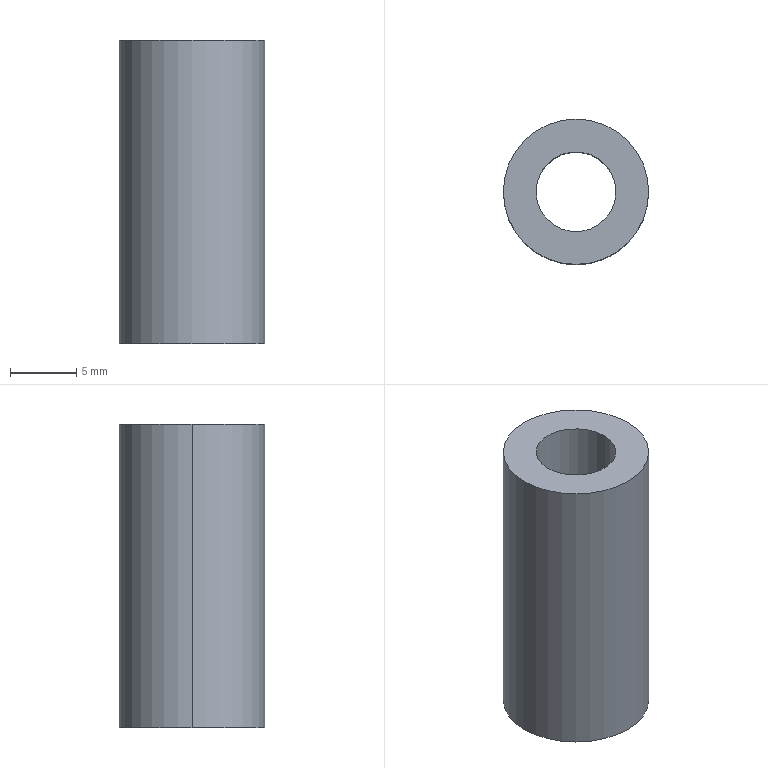Part | NX | features BREP 1 | 1 solid | 6 faces | box 11 x 11 x 23 mm | volume 1525 mm3 | cylinder 4 | plane 2 | commonest cylinder face diameters 6.05 x2 11 x2
STEP:
#1=CARTESIAN_POINT('',(2.513,-540.502,3.4));
#2=VERTEX_POINT('',#1);
#3=CARTESIAN_POINT('',(-3.537,-540.502,3.4));
#4=VERTEX_POINT('',#3);
#5=CARTESIAN_POINT('',(-0.5121,-540.502,3.4));
#6=DIRECTION('',(0.,0.,-1.));
#7=DIRECTION('',(1.,0.,0.));
#8=AXIS2_PLACEMENT_3D('',#5,#6,#7);
#9=CIRCLE('',#8,3.025);
#10=EDGE_CURVE('',#2,#4,#9,.T.);
#11=ORIENTED_EDGE('',*,*,#10,.T.);
#12=CARTESIAN_POINT('',(-3.537,-540.502,26.4));
#13=VERTEX_POINT('',#12);
#14=CARTESIAN_POINT('',(-3.537,-540.502,-16.2));
#15=DIRECTION('',(0.,0.,1.));
#16=VECTOR('',#15,1000.);
#17=LINE('',#14,#16);
#18=EDGE_CURVE('',#4,#13,#17,.T.);
#19=ORIENTED_EDGE('',*,*,#18,.T.);
#20=CARTESIAN_POINT('',(2.513,-540.502,26.4));
#21=VERTEX_POINT('',#20);
#22=CARTESIAN_POINT('',(-0.5121,-540.502,26.4));
#23=DIRECTION('',(0.,0.,1.));
#24=DIRECTION('',(-1.,0.,0.));
#25=AXIS2_PLACEMENT_3D('',#22,#23,#24);
#26=CIRCLE('',#25,3.025);
#27=EDGE_CURVE('',#13,#21,#26,.T.);
#28=ORIENTED_EDGE('',*,*,#27,.T.);
#29=CARTESIAN_POINT('',(2.513,-540.502,-16.2));
#30=DIRECTION('',(0.,0.,1.));
#31=VECTOR('',#30,1000.);
#32=LINE('',#29,#31);
#33=EDGE_CURVE('',#2,#21,#32,.T.);
#34=ORIENTED_EDGE('',*,*,#33,.F.);
#35=EDGE_LOOP('',(#11,#19,#28,#34));
#36=FACE_BOUND('',#35,.T.);
#37=CARTESIAN_POINT('',(-0.5121,-540.502,-16.2));
#38=DIRECTION('',(0.,0.,1.));
#39=DIRECTION('',(-1.,0.,0.));
#40=AXIS2_PLACEMENT_3D('',#37,#38,#39);
#41=CYLINDRICAL_SURFACE('',#40,3.025);
#42=ADVANCED_FACE('',(#36),#41,.F.);
#43=CARTESIAN_POINT('',(-6.012,-540.502,26.4));
#44=VERTEX_POINT('',#43);
#45=CARTESIAN_POINT('',(4.988,-540.502,26.4));
#46=VERTEX_POINT('',#45);
#47=CARTESIAN_POINT('',(-0.5121,-540.502,26.4));
#48=DIRECTION('',(0.,0.,-1.));
#49=DIRECTION('',(-1.,0.,0.));
#50=AXIS2_PLACEMENT_3D('',#47,#48,#49);
#51=CIRCLE('',#50,5.5);
#52=EDGE_CURVE('',#44,#46,#51,.T.);
#53=ORIENTED_EDGE('',*,*,#52,.T.);
#54=CARTESIAN_POINT('',(4.988,-540.502,3.4));
#55=VERTEX_POINT('',#54);
#56=CARTESIAN_POINT('',(4.988,-540.502,44.156));
#57=DIRECTION('',(0.,0.,-1.));
#58=VECTOR('',#57,1000.);
#59=LINE('',#56,#58);
#60=EDGE_CURVE('',#55,#46,#59,.F.);
#61=ORIENTED_EDGE('',*,*,#60,.F.);
#62=CARTESIAN_POINT('',(-6.012,-540.502,3.4));
#63=VERTEX_POINT('',#62);
#64=CARTESIAN_POINT('',(-0.5121,-540.502,3.4));
#65=DIRECTION('',(0.,0.,1.));
#66=DIRECTION('',(1.,0.,0.));
#67=AXIS2_PLACEMENT_3D('',#64,#65,#66);
#68=CIRCLE('',#67,5.5);
#69=EDGE_CURVE('',#55,#63,#68,.T.);
#70=ORIENTED_EDGE('',*,*,#69,.T.);
#71=CARTESIAN_POINT('',(-6.012,-540.502,44.156));
#72=DIRECTION('',(0.,0.,-1.));
#73=VECTOR('',#72,1000.);
#74=LINE('',#71,#73);
#75=EDGE_CURVE('',#63,#44,#74,.F.);
#76=ORIENTED_EDGE('',*,*,#75,.T.);
#77=EDGE_LOOP('',(#53,#61,#70,#76));
#78=FACE_BOUND('',#77,.T.);
#79=CARTESIAN_POINT('',(-0.5121,-540.502,44.156));
#80=DIRECTION('',(0.,0.,-1.));
#81=DIRECTION('',(1.,0.,0.));
#82=AXIS2_PLACEMENT_3D('',#79,#80,#81);
#83=CYLINDRICAL_SURFACE('',#82,5.5);
#84=ADVANCED_FACE('',(#78),#83,.T.);
#85=ORIENTED_EDGE('',*,*,#60,.T.);
#86=CARTESIAN_POINT('',(-0.5121,-540.502,26.4));
#87=DIRECTION('',(0.,0.,-1.));
#88=DIRECTION('',(-1.,0.,0.));
#89=AXIS2_PLACEMENT_3D('',#86,#87,#88);
#90=CIRCLE('',#89,5.5);
#91=EDGE_CURVE('',#46,#44,#90,.T.);
#92=ORIENTED_EDGE('',*,*,#91,.T.);
#93=ORIENTED_EDGE('',*,*,#75,.F.);
#94=CARTESIAN_POINT('',(-0.5121,-540.502,3.4));
#95=DIRECTION('',(0.,0.,1.));
#96=DIRECTION('',(1.,0.,0.));
#97=AXIS2_PLACEMENT_3D('',#94,#95,#96);
#98=CIRCLE('',#97,5.5);
#99=EDGE_CURVE('',#63,#55,#98,.T.);
#100=ORIENTED_EDGE('',*,*,#99,.T.);
#101=EDGE_LOOP('',(#85,#92,#93,#100));
#102=FACE_BOUND('',#101,.T.);
#103=CARTESIAN_POINT('',(-0.5121,-540.502,44.156));
#104=DIRECTION('',(0.,0.,-1.));
#105=DIRECTION('',(1.,0.,0.));
#106=AXIS2_PLACEMENT_3D('',#103,#104,#105);
#107=CYLINDRICAL_SURFACE('',#106,5.5);
#108=ADVANCED_FACE('',(#102),#107,.T.);
#109=ORIENTED_EDGE('',*,*,#18,.F.);
#110=CARTESIAN_POINT('',(-0.5121,-540.502,3.4));
#111=DIRECTION('',(0.,0.,-1.));
#112=DIRECTION('',(1.,0.,0.));
#113=AXIS2_PLACEMENT_3D('',#110,#111,#112);
#114=CIRCLE('',#113,3.025);
#115=EDGE_CURVE('',#4,#2,#114,.T.);
#116=ORIENTED_EDGE('',*,*,#115,.T.);
#117=ORIENTED_EDGE('',*,*,#33,.T.);
#118=CARTESIAN_POINT('',(-0.5121,-540.502,26.4));
#119=DIRECTION('',(0.,0.,1.));
#120=DIRECTION('',(-1.,0.,0.));
#121=AXIS2_PLACEMENT_3D('',#118,#119,#120);
#122=CIRCLE('',#121,3.025);
#123=EDGE_CURVE('',#21,#13,#122,.T.);
#124=ORIENTED_EDGE('',*,*,#123,.T.);
#125=EDGE_LOOP('',(#109,#116,#117,#124));
#126=FACE_BOUND('',#125,.T.);
#127=CARTESIAN_POINT('',(-0.5121,-540.502,-16.2));
#128=DIRECTION('',(0.,0.,1.));
#129=DIRECTION('',(-1.,0.,0.));
#130=AXIS2_PLACEMENT_3D('',#127,#128,#129);
#131=CYLINDRICAL_SURFACE('',#130,3.025);
#132=ADVANCED_FACE('',(#126),#131,.F.);
#133=ORIENTED_EDGE('',*,*,#52,.F.);
#134=ORIENTED_EDGE('',*,*,#91,.F.);
#135=EDGE_LOOP('',(#133,#134));
#136=FACE_BOUND('',#135,.T.);
#137=ORIENTED_EDGE('',*,*,#123,.F.);
#138=ORIENTED_EDGE('',*,*,#27,.F.);
#139=EDGE_LOOP('',(#137,#138));
#140=FACE_BOUND('',#139,.T.);
#141=CARTESIAN_POINT('',(-0.5121,-540.502,26.4));
#142=DIRECTION('',(0.,0.,-1.));
#143=DIRECTION('',(0.,1.,0.));
#144=AXIS2_PLACEMENT_3D('',#141,#142,#143);
#145=PLANE('',#144);
#146=ADVANCED_FACE('',(#136,#140),#145,.F.);
#147=ORIENTED_EDGE('',*,*,#99,.F.);
#148=ORIENTED_EDGE('',*,*,#69,.F.);
#149=EDGE_LOOP('',(#147,#148));
#150=FACE_BOUND('',#149,.T.);
#151=ORIENTED_EDGE('',*,*,#10,.F.);
#152=ORIENTED_EDGE('',*,*,#115,.F.);
#153=EDGE_LOOP('',(#151,#152));
#154=FACE_BOUND('',#153,.T.);
#155=CARTESIAN_POINT('',(-0.5121,-540.502,3.4));
#156=DIRECTION('',(0.,0.,1.));
#157=DIRECTION('',(-1.,0.,0.));
#158=AXIS2_PLACEMENT_3D('',#155,#156,#157);
#159=PLANE('',#158);
#160=ADVANCED_FACE('',(#150,#154),#159,.F.);
#161=CLOSED_SHELL('',(#42,#84,#108,#132,#146,#160));
#162=MANIFOLD_SOLID_BREP('',#161);
#163=(LENGTH_UNIT()NAMED_UNIT(*)SI_UNIT(.MILLI.,.METRE.));
#164=UNCERTAINTY_MEASURE_WITH_UNIT(LENGTH_MEASURE(0.00001),#163,'','');
#165=(NAMED_UNIT(*)PLANE_ANGLE_UNIT()SI_UNIT($,.RADIAN.));
#166=(NAMED_UNIT(*)SI_UNIT($,.STERADIAN.)SOLID_ANGLE_UNIT());
#167=(GEOMETRIC_REPRESENTATION_CONTEXT(3)GLOBAL_UNCERTAINTY_ASSIGNED_CONTEXT((#164))GLOBAL_UNIT_ASSIGNED_CONTEXT((#163,#165,#166))REPRESENTATION_CONTEXT('',''));
#168=ADVANCED_BREP_SHAPE_REPRESENTATION('',(#162),#167);